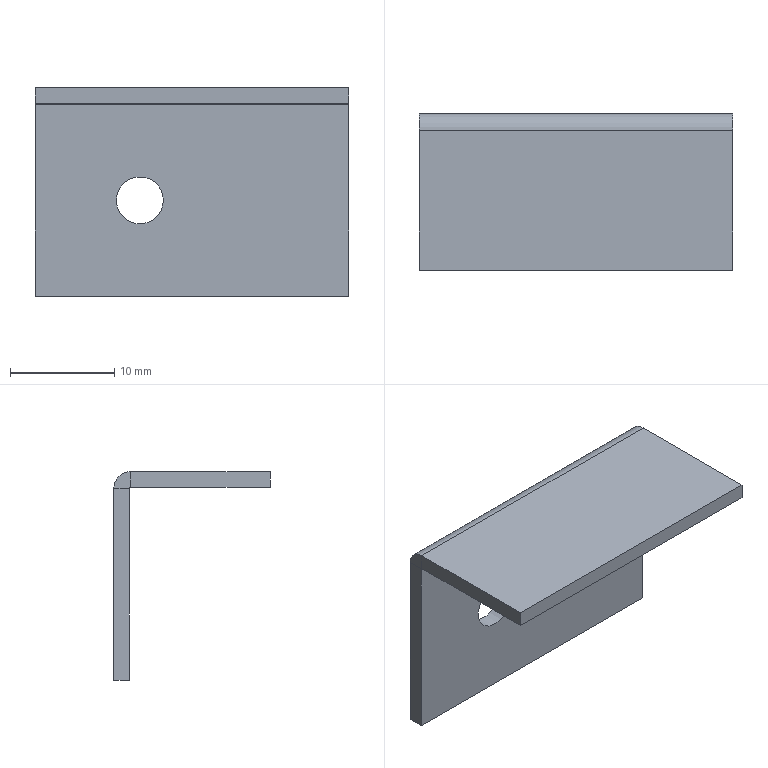Part | SolidWorks | features SplitBody 1 | 1 solid | 16 faces | box 30 x 15 x 20 mm | volume 1467 mm3 | plane 12 | cylinder 4 | commonest cylinder face diameters 4.5 x2 0.2 x1 3.2 x1
STEP:
#1=CARTESIAN_POINT('',(9.45,1360.8,288.));
#2=VERTEX_POINT('',#1);
#3=CARTESIAN_POINT('',(13.95,1360.8,288.));
#4=VERTEX_POINT('',#3);
#5=CARTESIAN_POINT('',(11.7,1360.8,288.));
#6=DIRECTION('',(0.,-1.,0.));
#7=DIRECTION('',(1.,0.,0.));
#8=AXIS2_PLACEMENT_3D('',#5,#6,#7);
#9=CIRCLE('',#8,2.25);
#10=EDGE_CURVE('',#2,#4,#9,.T.);
#11=ORIENTED_EDGE('',*,*,#10,.T.);
#12=CARTESIAN_POINT('',(13.95,1362.3,288.));
#13=VERTEX_POINT('',#12);
#14=CARTESIAN_POINT('',(13.95,1357.3,288.));
#15=DIRECTION('',(0.,1.,0.));
#16=VECTOR('',#15,1000.);
#17=LINE('',#14,#16);
#18=EDGE_CURVE('',#4,#13,#17,.T.);
#19=ORIENTED_EDGE('',*,*,#18,.T.);
#20=CARTESIAN_POINT('',(9.45,1362.3,288.));
#21=VERTEX_POINT('',#20);
#22=CARTESIAN_POINT('',(11.7,1362.3,288.));
#23=DIRECTION('',(0.,1.,0.));
#24=DIRECTION('',(-1.,0.,0.));
#25=AXIS2_PLACEMENT_3D('',#22,#23,#24);
#26=CIRCLE('',#25,2.25);
#27=EDGE_CURVE('',#13,#21,#26,.T.);
#28=ORIENTED_EDGE('',*,*,#27,.T.);
#29=CARTESIAN_POINT('',(9.45,1357.3,288.));
#30=DIRECTION('',(0.,1.,0.));
#31=VECTOR('',#30,1000.);
#32=LINE('',#29,#31);
#33=EDGE_CURVE('',#2,#21,#32,.T.);
#34=ORIENTED_EDGE('',*,*,#33,.F.);
#35=EDGE_LOOP('',(#11,#19,#28,#34));
#36=FACE_OUTER_BOUND('',#35,.T.);
#37=CARTESIAN_POINT('',(11.7,1357.3,288.));
#38=DIRECTION('',(0.,1.,0.));
#39=DIRECTION('',(-1.,0.,0.));
#40=AXIS2_PLACEMENT_3D('',#37,#38,#39);
#41=CYLINDRICAL_SURFACE('',#40,2.25);
#42=ADVANCED_FACE('',(#36),#41,.F.);
#43=CARTESIAN_POINT('',(31.7,1362.3,297.2));
#44=VERTEX_POINT('',#43);
#45=CARTESIAN_POINT('',(31.7,1360.8,297.2));
#46=VERTEX_POINT('',#45);
#47=CARTESIAN_POINT('',(31.7,1362.3,297.2));
#48=DIRECTION('',(0.,-1.,0.));
#49=VECTOR('',#48,1000.);
#50=LINE('',#47,#49);
#51=EDGE_CURVE('',#44,#46,#50,.T.);
#52=ORIENTED_EDGE('',*,*,#51,.F.);
#53=CARTESIAN_POINT('',(31.7,1360.7,298.8));
#54=VERTEX_POINT('',#53);
#55=CARTESIAN_POINT('',(31.7,1360.7,297.2));
#56=DIRECTION('',(1.,0.,0.));
#57=DIRECTION('',(0.,-1.,0.));
#58=AXIS2_PLACEMENT_3D('',#55,#56,#57);
#59=CIRCLE('',#58,1.6);
#60=EDGE_CURVE('',#44,#54,#59,.T.);
#61=ORIENTED_EDGE('',*,*,#60,.T.);
#62=CARTESIAN_POINT('',(31.7,1360.7,297.3));
#63=VERTEX_POINT('',#62);
#64=CARTESIAN_POINT('',(31.7,1360.7,297.3));
#65=DIRECTION('',(0.,0.,1.));
#66=VECTOR('',#65,1000.);
#67=LINE('',#64,#66);
#68=EDGE_CURVE('',#63,#54,#67,.T.);
#69=ORIENTED_EDGE('',*,*,#68,.F.);
#70=CARTESIAN_POINT('',(31.7,1360.7,297.2));
#71=DIRECTION('',(1.,0.,0.));
#72=DIRECTION('',(0.,0.,-1.));
#73=AXIS2_PLACEMENT_3D('',#70,#71,#72);
#74=CIRCLE('',#73,0.1);
#75=EDGE_CURVE('',#46,#63,#74,.T.);
#76=ORIENTED_EDGE('',*,*,#75,.F.);
#77=EDGE_LOOP('',(#52,#61,#69,#76));
#78=FACE_OUTER_BOUND('',#77,.T.);
#79=CARTESIAN_POINT('',(31.7,1362.3,297.2));
#80=DIRECTION('',(1.,0.,0.));
#81=DIRECTION('',(0.,1.,0.));
#82=AXIS2_PLACEMENT_3D('',#79,#80,#81);
#83=PLANE('',#82);
#84=ADVANCED_FACE('',(#78),#83,.T.);
#85=CARTESIAN_POINT('',(31.7,1362.3,278.8));
#86=VERTEX_POINT('',#85);
#87=CARTESIAN_POINT('',(31.7,1362.3,278.8));
#88=DIRECTION('',(0.,0.,1.));
#89=VECTOR('',#88,1000.);
#90=LINE('',#87,#89);
#91=EDGE_CURVE('',#86,#44,#90,.T.);
#92=ORIENTED_EDGE('',*,*,#91,.T.);
#93=ORIENTED_EDGE('',*,*,#51,.T.);
#94=CARTESIAN_POINT('',(31.7,1360.8,278.8));
#95=VERTEX_POINT('',#94);
#96=CARTESIAN_POINT('',(31.7,1360.8,278.8));
#97=DIRECTION('',(0.,0.,1.));
#98=VECTOR('',#97,1000.);
#99=LINE('',#96,#98);
#100=EDGE_CURVE('',#95,#46,#99,.T.);
#101=ORIENTED_EDGE('',*,*,#100,.F.);
#102=CARTESIAN_POINT('',(31.7,1362.3,278.8));
#103=DIRECTION('',(0.,-1.,0.));
#104=VECTOR('',#103,1000.);
#105=LINE('',#102,#104);
#106=EDGE_CURVE('',#86,#95,#105,.T.);
#107=ORIENTED_EDGE('',*,*,#106,.F.);
#108=EDGE_LOOP('',(#92,#93,#101,#107));
#109=FACE_OUTER_BOUND('',#108,.T.);
#110=CARTESIAN_POINT('',(31.7,1360.7,297.3));
#111=DIRECTION('',(1.,0.,0.));
#112=DIRECTION('',(0.,1.,0.));
#113=AXIS2_PLACEMENT_3D('',#110,#111,#112);
#114=PLANE('',#113);
#115=ADVANCED_FACE('',(#109),#114,.T.);
#116=CARTESIAN_POINT('',(1.7,1360.7,298.8));
#117=VERTEX_POINT('',#116);
#118=CARTESIAN_POINT('',(1.7,1360.7,297.3));
#119=VERTEX_POINT('',#118);
#120=CARTESIAN_POINT('',(1.7,1360.7,298.8));
#121=DIRECTION('',(0.,0.,-1.));
#122=VECTOR('',#121,1000.);
#123=LINE('',#120,#122);
#124=EDGE_CURVE('',#117,#119,#123,.T.);
#125=ORIENTED_EDGE('',*,*,#124,.F.);
#126=CARTESIAN_POINT('',(1.7,1362.3,297.2));
#127=VERTEX_POINT('',#126);
#128=CARTESIAN_POINT('',(1.7,1360.7,297.2));
#129=DIRECTION('',(1.,0.,0.));
#130=DIRECTION('',(0.,-1.,0.));
#131=AXIS2_PLACEMENT_3D('',#128,#129,#130);
#132=CIRCLE('',#131,1.6);
#133=EDGE_CURVE('',#127,#117,#132,.T.);
#134=ORIENTED_EDGE('',*,*,#133,.F.);
#135=CARTESIAN_POINT('',(1.7,1360.8,297.2));
#136=VERTEX_POINT('',#135);
#137=CARTESIAN_POINT('',(1.7,1360.8,297.2));
#138=DIRECTION('',(0.,1.,0.));
#139=VECTOR('',#138,1000.);
#140=LINE('',#137,#139);
#141=EDGE_CURVE('',#136,#127,#140,.T.);
#142=ORIENTED_EDGE('',*,*,#141,.F.);
#143=CARTESIAN_POINT('',(1.7,1360.7,297.2));
#144=DIRECTION('',(1.,0.,0.));
#145=DIRECTION('',(0.,0.,-1.));
#146=AXIS2_PLACEMENT_3D('',#143,#144,#145);
#147=CIRCLE('',#146,0.1);
#148=EDGE_CURVE('',#136,#119,#147,.T.);
#149=ORIENTED_EDGE('',*,*,#148,.T.);
#150=EDGE_LOOP('',(#125,#134,#142,#149));
#151=FACE_OUTER_BOUND('',#150,.T.);
#152=CARTESIAN_POINT('',(1.7,1360.7,298.8));
#153=DIRECTION('',(-1.,0.,0.));
#154=DIRECTION('',(0.,-1.,0.));
#155=AXIS2_PLACEMENT_3D('',#152,#153,#154);
#156=PLANE('',#155);
#157=ADVANCED_FACE('',(#151),#156,.T.);
#158=CARTESIAN_POINT('',(1.7,1347.3,298.8));
#159=VERTEX_POINT('',#158);
#160=CARTESIAN_POINT('',(1.7,1362.3,298.8));
#161=DIRECTION('',(0.,-1.,0.));
#162=VECTOR('',#161,1000.);
#163=LINE('',#160,#162);
#164=EDGE_CURVE('',#117,#159,#163,.T.);
#165=ORIENTED_EDGE('',*,*,#164,.F.);
#166=ORIENTED_EDGE('',*,*,#124,.T.);
#167=CARTESIAN_POINT('',(1.7,1347.3,297.3));
#168=VERTEX_POINT('',#167);
#169=CARTESIAN_POINT('',(1.7,1362.3,297.3));
#170=DIRECTION('',(0.,-1.,0.));
#171=VECTOR('',#170,1000.);
#172=LINE('',#169,#171);
#173=EDGE_CURVE('',#119,#168,#172,.T.);
#174=ORIENTED_EDGE('',*,*,#173,.T.);
#175=CARTESIAN_POINT('',(1.7,1347.3,297.3));
#176=DIRECTION('',(0.,0.,1.));
#177=VECTOR('',#176,1000.);
#178=LINE('',#175,#177);
#179=EDGE_CURVE('',#168,#159,#178,.T.);
#180=ORIENTED_EDGE('',*,*,#179,.T.);
#181=EDGE_LOOP('',(#165,#166,#174,#180));
#182=FACE_OUTER_BOUND('',#181,.T.);
#183=CARTESIAN_POINT('',(1.7,1360.8,297.2));
#184=DIRECTION('',(-1.,0.,0.));
#185=DIRECTION('',(0.,-1.,0.));
#186=AXIS2_PLACEMENT_3D('',#183,#184,#185);
#187=PLANE('',#186);
#188=ADVANCED_FACE('',(#182),#187,.T.);
#189=ORIENTED_EDGE('',*,*,#164,.T.);
#190=CARTESIAN_POINT('',(31.7,1347.3,298.8));
#191=VERTEX_POINT('',#190);
#192=CARTESIAN_POINT('',(31.7,1347.3,298.8));
#193=DIRECTION('',(-1.,0.,0.));
#194=VECTOR('',#193,1000.);
#195=LINE('',#192,#194);
#196=EDGE_CURVE('',#191,#159,#195,.T.);
#197=ORIENTED_EDGE('',*,*,#196,.F.);
#198=CARTESIAN_POINT('',(31.7,1362.3,298.8));
#199=DIRECTION('',(0.,-1.,0.));
#200=VECTOR('',#199,1000.);
#201=LINE('',#198,#200);
#202=EDGE_CURVE('',#54,#191,#201,.T.);
#203=ORIENTED_EDGE('',*,*,#202,.F.);
#204=CARTESIAN_POINT('',(31.7,1360.7,298.8));
#205=DIRECTION('',(-1.,0.,0.));
#206=VECTOR('',#205,1000.);
#207=LINE('',#204,#206);
#208=EDGE_CURVE('',#54,#117,#207,.T.);
#209=ORIENTED_EDGE('',*,*,#208,.T.);
#210=EDGE_LOOP('',(#189,#197,#203,#209));
#211=FACE_OUTER_BOUND('',#210,.T.);
#212=CARTESIAN_POINT('',(31.7,1362.3,298.8));
#213=DIRECTION('',(0.,0.,-1.));
#214=DIRECTION('',(-1.,0.,0.));
#215=AXIS2_PLACEMENT_3D('',#212,#213,#214);
#216=PLANE('',#215);
#217=ADVANCED_FACE('',(#211),#216,.F.);
#218=ORIENTED_EDGE('',*,*,#179,.F.);
#219=CARTESIAN_POINT('',(31.7,1347.3,297.3));
#220=VERTEX_POINT('',#219);
#221=CARTESIAN_POINT('',(31.7,1347.3,297.3));
#222=DIRECTION('',(-1.,0.,0.));
#223=VECTOR('',#222,1000.);
#224=LINE('',#221,#223);
#225=EDGE_CURVE('',#220,#168,#224,.T.);
#226=ORIENTED_EDGE('',*,*,#225,.F.);
#227=CARTESIAN_POINT('',(31.7,1347.3,297.3));
#228=DIRECTION('',(0.,0.,1.));
#229=VECTOR('',#228,1000.);
#230=LINE('',#227,#229);
#231=EDGE_CURVE('',#220,#191,#230,.T.);
#232=ORIENTED_EDGE('',*,*,#231,.T.);
#233=ORIENTED_EDGE('',*,*,#196,.T.);
#234=EDGE_LOOP('',(#218,#226,#232,#233));
#235=FACE_OUTER_BOUND('',#234,.T.);
#236=CARTESIAN_POINT('',(31.7,1347.3,297.3));
#237=DIRECTION('',(0.,-1.,0.));
#238=DIRECTION('',(1.,0.,0.));
#239=AXIS2_PLACEMENT_3D('',#236,#237,#238);
#240=PLANE('',#239);
#241=ADVANCED_FACE('',(#235),#240,.T.);
#242=ORIENTED_EDGE('',*,*,#173,.F.);
#243=CARTESIAN_POINT('',(31.7,1360.7,297.3));
#244=DIRECTION('',(-1.,0.,0.));
#245=VECTOR('',#244,1000.);
#246=LINE('',#243,#245);
#247=EDGE_CURVE('',#63,#119,#246,.T.);
#248=ORIENTED_EDGE('',*,*,#247,.F.);
#249=CARTESIAN_POINT('',(31.7,1362.3,297.3));
#250=DIRECTION('',(0.,-1.,0.));
#251=VECTOR('',#250,1000.);
#252=LINE('',#249,#251);
#253=EDGE_CURVE('',#63,#220,#252,.T.);
#254=ORIENTED_EDGE('',*,*,#253,.T.);
#255=ORIENTED_EDGE('',*,*,#225,.T.);
#256=EDGE_LOOP('',(#242,#248,#254,#255));
#257=FACE_OUTER_BOUND('',#256,.T.);
#258=CARTESIAN_POINT('',(31.7,1362.3,297.3));
#259=DIRECTION('',(0.,0.,-1.));
#260=DIRECTION('',(-1.,0.,0.));
#261=AXIS2_PLACEMENT_3D('',#258,#259,#260);
#262=PLANE('',#261);
#263=ADVANCED_FACE('',(#257),#262,.T.);
#264=ORIENTED_EDGE('',*,*,#148,.F.);
#265=CARTESIAN_POINT('',(31.7,1360.8,297.2));
#266=DIRECTION('',(-1.,0.,0.));
#267=VECTOR('',#266,1000.);
#268=LINE('',#265,#267);
#269=EDGE_CURVE('',#46,#136,#268,.T.);
#270=ORIENTED_EDGE('',*,*,#269,.F.);
#271=ORIENTED_EDGE('',*,*,#75,.T.);
#272=ORIENTED_EDGE('',*,*,#247,.T.);
#273=EDGE_LOOP('',(#264,#270,#271,#272));
#274=FACE_OUTER_BOUND('',#273,.T.);
#275=CARTESIAN_POINT('',(31.7,1360.7,297.2));
#276=DIRECTION('',(-1.,0.,0.));
#277=DIRECTION('',(0.,-1.,0.));
#278=AXIS2_PLACEMENT_3D('',#275,#276,#277);
#279=CYLINDRICAL_SURFACE('',#278,0.1);
#280=ADVANCED_FACE('',(#274),#279,.F.);
#281=ORIENTED_EDGE('',*,*,#10,.F.);
#282=CARTESIAN_POINT('',(11.7,1360.8,288.));
#283=DIRECTION('',(0.,-1.,0.));
#284=DIRECTION('',(1.,0.,0.));
#285=AXIS2_PLACEMENT_3D('',#282,#283,#284);
#286=CIRCLE('',#285,2.25);
#287=EDGE_CURVE('',#4,#2,#286,.T.);
#288=ORIENTED_EDGE('',*,*,#287,.F.);
#289=EDGE_LOOP('',(#281,#288));
#290=FACE_BOUND('',#289,.T.);
#291=CARTESIAN_POINT('',(1.7,1360.8,278.8));
#292=VERTEX_POINT('',#291);
#293=CARTESIAN_POINT('',(1.7,1360.8,278.8));
#294=DIRECTION('',(0.,0.,1.));
#295=VECTOR('',#294,1000.);
#296=LINE('',#293,#295);
#297=EDGE_CURVE('',#292,#136,#296,.T.);
#298=ORIENTED_EDGE('',*,*,#297,.F.);
#299=CARTESIAN_POINT('',(31.7,1360.8,278.8));
#300=DIRECTION('',(-1.,0.,0.));
#301=VECTOR('',#300,1000.);
#302=LINE('',#299,#301);
#303=EDGE_CURVE('',#95,#292,#302,.T.);
#304=ORIENTED_EDGE('',*,*,#303,.F.);
#305=ORIENTED_EDGE('',*,*,#100,.T.);
#306=ORIENTED_EDGE('',*,*,#269,.T.);
#307=EDGE_LOOP('',(#298,#304,#305,#306));
#308=FACE_OUTER_BOUND('',#307,.T.);
#309=CARTESIAN_POINT('',(31.7,1360.8,278.8));
#310=DIRECTION('',(0.,-1.,0.));
#311=DIRECTION('',(1.,0.,0.));
#312=AXIS2_PLACEMENT_3D('',#309,#310,#311);
#313=PLANE('',#312);
#314=ADVANCED_FACE('',(#290,#308),#313,.T.);
#315=CARTESIAN_POINT('',(1.7,1362.3,278.8));
#316=VERTEX_POINT('',#315);
#317=CARTESIAN_POINT('',(1.7,1362.3,278.8));
#318=DIRECTION('',(0.,-1.,0.));
#319=VECTOR('',#318,1000.);
#320=LINE('',#317,#319);
#321=EDGE_CURVE('',#316,#292,#320,.T.);
#322=ORIENTED_EDGE('',*,*,#321,.F.);
#323=CARTESIAN_POINT('',(31.7,1362.3,278.8));
#324=DIRECTION('',(-1.,0.,0.));
#325=VECTOR('',#324,1000.);
#326=LINE('',#323,#325);
#327=EDGE_CURVE('',#86,#316,#326,.T.);
#328=ORIENTED_EDGE('',*,*,#327,.F.);
#329=ORIENTED_EDGE('',*,*,#106,.T.);
#330=ORIENTED_EDGE('',*,*,#303,.T.);
#331=EDGE_LOOP('',(#322,#328,#329,#330));
#332=FACE_OUTER_BOUND('',#331,.T.);
#333=CARTESIAN_POINT('',(31.7,1362.3,278.8));
#334=DIRECTION('',(0.,0.,-1.));
#335=DIRECTION('',(-1.,0.,0.));
#336=AXIS2_PLACEMENT_3D('',#333,#334,#335);
#337=PLANE('',#336);
#338=ADVANCED_FACE('',(#332),#337,.T.);
#339=CARTESIAN_POINT('',(11.7,1362.3,288.));
#340=DIRECTION('',(0.,1.,0.));
#341=DIRECTION('',(-1.,0.,0.));
#342=AXIS2_PLACEMENT_3D('',#339,#340,#341);
#343=CIRCLE('',#342,2.25);
#344=EDGE_CURVE('',#21,#13,#343,.T.);
#345=ORIENTED_EDGE('',*,*,#344,.F.);
#346=ORIENTED_EDGE('',*,*,#27,.F.);
#347=EDGE_LOOP('',(#345,#346));
#348=FACE_BOUND('',#347,.T.);
#349=CARTESIAN_POINT('',(1.7,1362.3,278.8));
#350=DIRECTION('',(0.,0.,1.));
#351=VECTOR('',#350,1000.);
#352=LINE('',#349,#351);
#353=EDGE_CURVE('',#316,#127,#352,.T.);
#354=ORIENTED_EDGE('',*,*,#353,.T.);
#355=CARTESIAN_POINT('',(31.7,1362.3,297.2));
#356=DIRECTION('',(-1.,0.,0.));
#357=VECTOR('',#356,1000.);
#358=LINE('',#355,#357);
#359=EDGE_CURVE('',#44,#127,#358,.T.);
#360=ORIENTED_EDGE('',*,*,#359,.F.);
#361=ORIENTED_EDGE('',*,*,#91,.F.);
#362=ORIENTED_EDGE('',*,*,#327,.T.);
#363=EDGE_LOOP('',(#354,#360,#361,#362));
#364=FACE_OUTER_BOUND('',#363,.T.);
#365=CARTESIAN_POINT('',(31.7,1362.3,278.8));
#366=DIRECTION('',(0.,-1.,0.));
#367=DIRECTION('',(1.,0.,0.));
#368=AXIS2_PLACEMENT_3D('',#365,#366,#367);
#369=PLANE('',#368);
#370=ADVANCED_FACE('',(#348,#364),#369,.F.);
#371=ORIENTED_EDGE('',*,*,#133,.T.);
#372=ORIENTED_EDGE('',*,*,#208,.F.);
#373=ORIENTED_EDGE('',*,*,#60,.F.);
#374=ORIENTED_EDGE('',*,*,#359,.T.);
#375=EDGE_LOOP('',(#371,#372,#373,#374));
#376=FACE_OUTER_BOUND('',#375,.T.);
#377=CARTESIAN_POINT('',(31.7,1360.7,297.2));
#378=DIRECTION('',(-1.,0.,0.));
#379=DIRECTION('',(0.,-1.,0.));
#380=AXIS2_PLACEMENT_3D('',#377,#378,#379);
#381=CYLINDRICAL_SURFACE('',#380,1.6);
#382=ADVANCED_FACE('',(#376),#381,.T.);
#383=ORIENTED_EDGE('',*,*,#202,.T.);
#384=ORIENTED_EDGE('',*,*,#231,.F.);
#385=ORIENTED_EDGE('',*,*,#253,.F.);
#386=ORIENTED_EDGE('',*,*,#68,.T.);
#387=EDGE_LOOP('',(#383,#384,#385,#386));
#388=FACE_OUTER_BOUND('',#387,.T.);
#389=CARTESIAN_POINT('',(31.7,1360.7,297.2));
#390=DIRECTION('',(1.,0.,0.));
#391=DIRECTION('',(0.,0.,-1.));
#392=AXIS2_PLACEMENT_3D('',#389,#390,#391);
#393=PLANE('',#392);
#394=ADVANCED_FACE('',(#388),#393,.T.);
#395=ORIENTED_EDGE('',*,*,#297,.T.);
#396=ORIENTED_EDGE('',*,*,#141,.T.);
#397=ORIENTED_EDGE('',*,*,#353,.F.);
#398=ORIENTED_EDGE('',*,*,#321,.T.);
#399=EDGE_LOOP('',(#395,#396,#397,#398));
#400=FACE_OUTER_BOUND('',#399,.T.);
#401=CARTESIAN_POINT('',(1.7,1360.7,297.2));
#402=DIRECTION('',(1.,0.,0.));
#403=DIRECTION('',(0.,0.,-1.));
#404=AXIS2_PLACEMENT_3D('',#401,#402,#403);
#405=PLANE('',#404);
#406=ADVANCED_FACE('',(#400),#405,.F.);
#407=ORIENTED_EDGE('',*,*,#18,.F.);
#408=ORIENTED_EDGE('',*,*,#287,.T.);
#409=ORIENTED_EDGE('',*,*,#33,.T.);
#410=ORIENTED_EDGE('',*,*,#344,.T.);
#411=EDGE_LOOP('',(#407,#408,#409,#410));
#412=FACE_OUTER_BOUND('',#411,.T.);
#413=CARTESIAN_POINT('',(11.7,1357.3,288.));
#414=DIRECTION('',(0.,1.,0.));
#415=DIRECTION('',(-1.,0.,0.));
#416=AXIS2_PLACEMENT_3D('',#413,#414,#415);
#417=CYLINDRICAL_SURFACE('',#416,2.25);
#418=ADVANCED_FACE('',(#412),#417,.F.);
#419=CLOSED_SHELL('',(#42,#84,#115,#157,#188,#217,#241,#263,#280,#314,#338,#370,#382,#394,#406,#418));
#420=MANIFOLD_SOLID_BREP('',#419);
#421=CARTESIAN_POINT('',(0.,0.,0.));
#422=DIRECTION('',(0.,0.,1.));
#423=DIRECTION('',(1.,0.,0.));
#424=AXIS2_PLACEMENT_3D('',#421,#422,#423);
#425=(LENGTH_UNIT()NAMED_UNIT(*)SI_UNIT(.MILLI.,.METRE.));
#426=UNCERTAINTY_MEASURE_WITH_UNIT(LENGTH_MEASURE(0.00001),#425,'','');
#427=(NAMED_UNIT(*)PLANE_ANGLE_UNIT()SI_UNIT($,.RADIAN.));
#428=(NAMED_UNIT(*)SI_UNIT($,.STERADIAN.)SOLID_ANGLE_UNIT());
#429=(GEOMETRIC_REPRESENTATION_CONTEXT(3)GLOBAL_UNCERTAINTY_ASSIGNED_CONTEXT((#426))GLOBAL_UNIT_ASSIGNED_CONTEXT((#425,#427,#428))REPRESENTATION_CONTEXT('',''));
#430=ADVANCED_BREP_SHAPE_REPRESENTATION('',(#420,#424),#429);